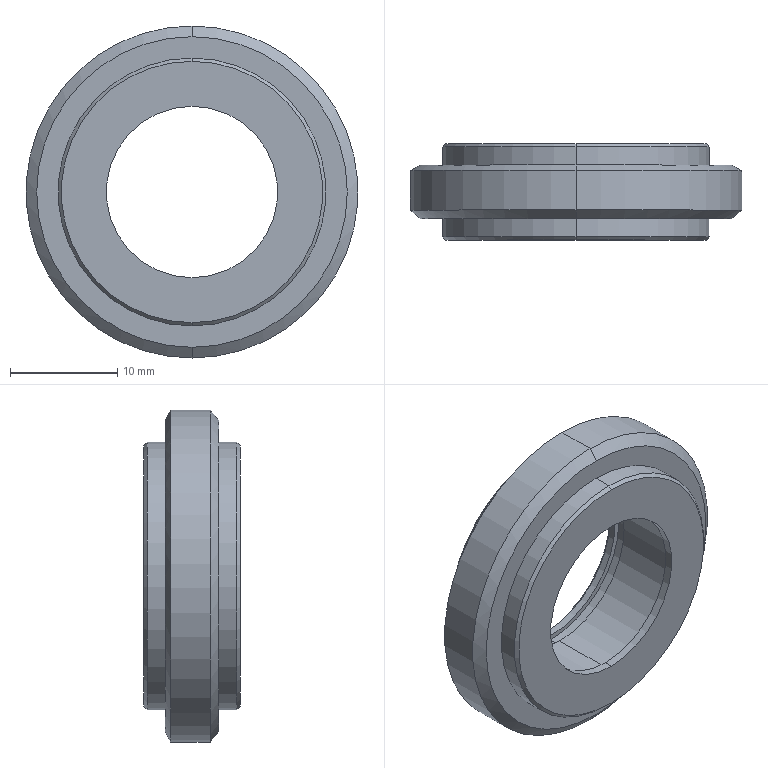Part | STEP file | 1 solid | 31 faces | box 31 x 9 x 31 mm | volume 3611 mm3 | cylinder 14 | cone 10 | plane 7 | commonest cylinder face diameters 17 x4 25 x4 16 x2 18 x2 31 x2